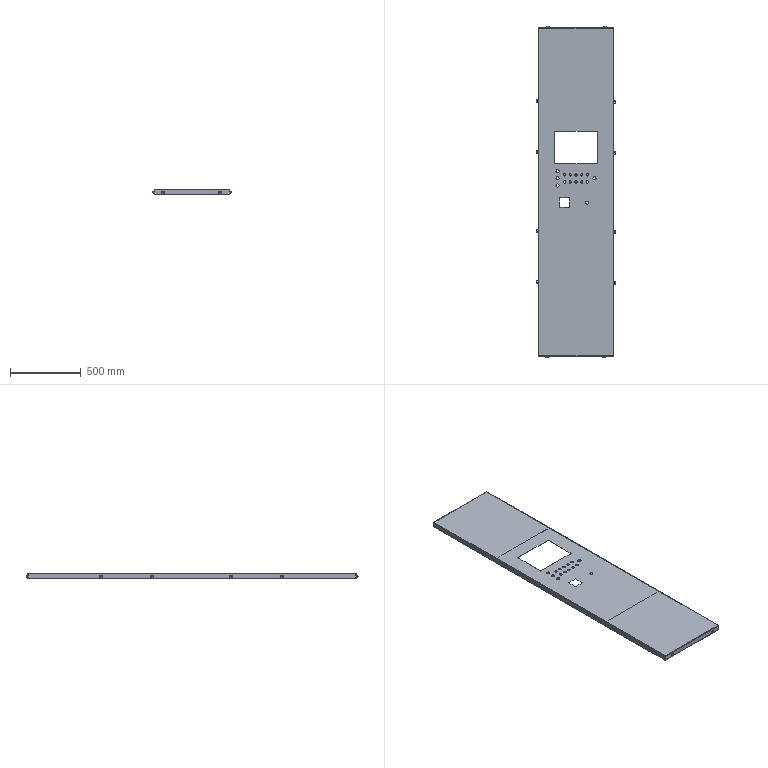Part | SolidWorks | features ReferencePattern 12, LocalLPattern 3 | 25 solids | 847 faces | box 560.594 x 2339 x 38 mm | volume 2295468 mm3 | plane 373 | cylinder 278 | cone 132 | spline 64 | commonest cylinder face diameters 20.854 x96 1.6 x36 4.917 x24 6 x24 6.6 x24 10 x24